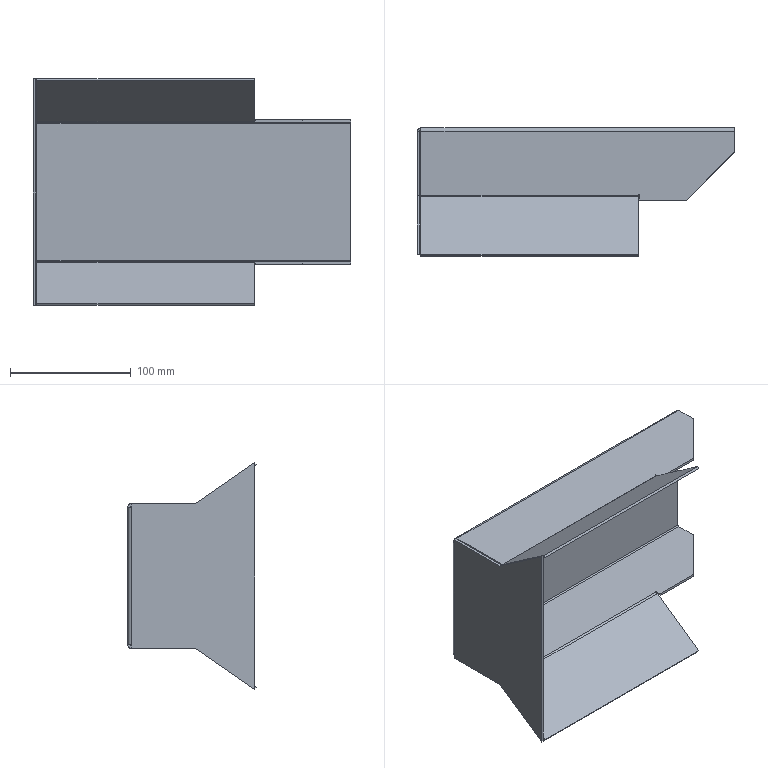Part | SolidWorks | features BaseBody 1 | 1 solid | 46 faces | box 263 x 106.293 x 188.106 mm | volume 187834 mm3 | plane 36 | cylinder 10 | commonest cylinder face diameters 2 x5 6 x5
STEP:
#1=CARTESIAN_POINT('',(-140.,-60.,118.));
#2=VERTEX_POINT('',#1);
#3=CARTESIAN_POINT('',(-100.,-20.,118.));
#4=VERTEX_POINT('',#3);
#5=CARTESIAN_POINT('',(-40.,40.,118.));
#6=DIRECTION('',(0.7071,0.7071,0.));
#7=VECTOR('',#6,1000.);
#8=LINE('',#5,#7);
#9=EDGE_CURVE('',#2,#4,#8,.T.);
#10=ORIENTED_EDGE('',*,*,#9,.T.);
#11=CARTESIAN_POINT('',(-100.,-20.,120.));
#12=VERTEX_POINT('',#11);
#13=CARTESIAN_POINT('',(-100.,-20.,272.315));
#14=DIRECTION('',(0.,0.,-1.));
#15=VECTOR('',#14,1000.);
#16=LINE('',#13,#15);
#17=EDGE_CURVE('',#12,#4,#16,.T.);
#18=ORIENTED_EDGE('',*,*,#17,.F.);
#19=CARTESIAN_POINT('',(-140.,-60.,120.));
#20=VERTEX_POINT('',#19);
#21=CARTESIAN_POINT('',(-140.,-60.,120.));
#22=DIRECTION('',(-0.7071,-0.7071,0.));
#23=VECTOR('',#22,1000.);
#24=LINE('',#21,#23);
#25=EDGE_CURVE('',#12,#20,#24,.T.);
#26=ORIENTED_EDGE('',*,*,#25,.T.);
#27=CARTESIAN_POINT('',(-140.,-60.,272.315));
#28=DIRECTION('',(0.,0.,-1.));
#29=VECTOR('',#28,1000.);
#30=LINE('',#27,#29);
#31=EDGE_CURVE('',#20,#2,#30,.T.);
#32=ORIENTED_EDGE('',*,*,#31,.T.);
#33=EDGE_LOOP('',(#10,#18,#26,#32));
#34=FACE_OUTER_BOUND('',#33,.T.);
#35=CARTESIAN_POINT('',(-140.,-60.,272.315));
#36=DIRECTION('',(-0.7071,0.7071,0.));
#37=DIRECTION('',(0.,0.,1.));
#38=AXIS2_PLACEMENT_3D('',#35,#36,#37);
#39=PLANE('',#38);
#40=ADVANCED_FACE('',(#34),#39,.F.);
#41=CARTESIAN_POINT('',(-100.,-3.,0.));
#42=VERTEX_POINT('',#41);
#43=CARTESIAN_POINT('',(-100.,0.,3.));
#44=VERTEX_POINT('',#43);
#45=CARTESIAN_POINT('',(-100.,-3.,3.));
#46=DIRECTION('',(1.,0.,0.));
#47=DIRECTION('',(0.,0.,1.));
#48=AXIS2_PLACEMENT_3D('',#45,#46,#47);
#49=CIRCLE('',#48,3.);
#50=EDGE_CURVE('',#42,#44,#49,.T.);
#51=ORIENTED_EDGE('',*,*,#50,.T.);
#52=CARTESIAN_POINT('',(-100.,0.,117.));
#53=VERTEX_POINT('',#52);
#54=CARTESIAN_POINT('',(-100.,0.,272.315));
#55=DIRECTION('',(0.,0.,-1.));
#56=VECTOR('',#55,1000.);
#57=LINE('',#54,#56);
#58=EDGE_CURVE('',#53,#44,#57,.T.);
#59=ORIENTED_EDGE('',*,*,#58,.F.);
#60=CARTESIAN_POINT('',(-100.,-3.,120.));
#61=VERTEX_POINT('',#60);
#62=CARTESIAN_POINT('',(-100.,-3.,117.));
#63=DIRECTION('',(1.,0.,0.));
#64=DIRECTION('',(0.,0.,1.));
#65=AXIS2_PLACEMENT_3D('',#62,#63,#64);
#66=CIRCLE('',#65,3.);
#67=EDGE_CURVE('',#53,#61,#66,.T.);
#68=ORIENTED_EDGE('',*,*,#67,.T.);
#69=CARTESIAN_POINT('',(-100.,-20.,120.));
#70=DIRECTION('',(0.,-1.,0.));
#71=VECTOR('',#70,1000.);
#72=LINE('',#69,#71);
#73=EDGE_CURVE('',#61,#12,#72,.T.);
#74=ORIENTED_EDGE('',*,*,#73,.T.);
#75=ORIENTED_EDGE('',*,*,#17,.T.);
#76=CARTESIAN_POINT('',(-100.,-3.,118.));
#77=VERTEX_POINT('',#76);
#78=CARTESIAN_POINT('',(-100.,0.,118.));
#79=DIRECTION('',(0.,1.,0.));
#80=VECTOR('',#79,1000.);
#81=LINE('',#78,#80);
#82=EDGE_CURVE('',#4,#77,#81,.T.);
#83=ORIENTED_EDGE('',*,*,#82,.T.);
#84=CARTESIAN_POINT('',(-100.,-2.,117.));
#85=VERTEX_POINT('',#84);
#86=CARTESIAN_POINT('',(-100.,-3.,117.));
#87=DIRECTION('',(1.,0.,0.));
#88=DIRECTION('',(0.,0.,1.));
#89=AXIS2_PLACEMENT_3D('',#86,#87,#88);
#90=CIRCLE('',#89,1.);
#91=EDGE_CURVE('',#85,#77,#90,.T.);
#92=ORIENTED_EDGE('',*,*,#91,.F.);
#93=CARTESIAN_POINT('',(-100.,-2.,3.));
#94=VERTEX_POINT('',#93);
#95=CARTESIAN_POINT('',(-100.,-2.,0.));
#96=DIRECTION('',(0.,0.,-1.));
#97=VECTOR('',#96,1000.);
#98=LINE('',#95,#97);
#99=EDGE_CURVE('',#85,#94,#98,.T.);
#100=ORIENTED_EDGE('',*,*,#99,.T.);
#101=CARTESIAN_POINT('',(-100.,-3.,2.));
#102=VERTEX_POINT('',#101);
#103=CARTESIAN_POINT('',(-100.,-3.,3.));
#104=DIRECTION('',(1.,0.,0.));
#105=DIRECTION('',(0.,0.,1.));
#106=AXIS2_PLACEMENT_3D('',#103,#104,#105);
#107=CIRCLE('',#106,1.);
#108=EDGE_CURVE('',#102,#94,#107,.T.);
#109=ORIENTED_EDGE('',*,*,#108,.F.);
#110=CARTESIAN_POINT('',(-100.,-20.,2.));
#111=VERTEX_POINT('',#110);
#112=CARTESIAN_POINT('',(-100.,0.,2.));
#113=DIRECTION('',(0.,1.,0.));
#114=VECTOR('',#113,1000.);
#115=LINE('',#112,#114);
#116=EDGE_CURVE('',#111,#102,#115,.T.);
#117=ORIENTED_EDGE('',*,*,#116,.F.);
#118=CARTESIAN_POINT('',(-100.,-20.,0.));
#119=VERTEX_POINT('',#118);
#120=CARTESIAN_POINT('',(-100.,-20.,272.315));
#121=DIRECTION('',(0.,0.,-1.));
#122=VECTOR('',#121,1000.);
#123=LINE('',#120,#122);
#124=EDGE_CURVE('',#111,#119,#123,.T.);
#125=ORIENTED_EDGE('',*,*,#124,.T.);
#126=CARTESIAN_POINT('',(-100.,-20.,0.));
#127=DIRECTION('',(0.,1.,0.));
#128=VECTOR('',#127,1000.);
#129=LINE('',#126,#128);
#130=EDGE_CURVE('',#119,#42,#129,.T.);
#131=ORIENTED_EDGE('',*,*,#130,.T.);
#132=EDGE_LOOP('',(#51,#59,#68,#74,#75,#83,#92,#100,#109,#117,#125,#131));
#133=FACE_OUTER_BOUND('',#132,.T.);
#134=CARTESIAN_POINT('',(-100.,-20.,272.315));
#135=DIRECTION('',(-1.,0.,0.));
#136=DIRECTION('',(0.,1.,0.));
#137=AXIS2_PLACEMENT_3D('',#134,#135,#136);
#138=PLANE('',#137);
#139=ADVANCED_FACE('',(#133),#138,.F.);
#140=CARTESIAN_POINT('',(-140.,-60.,2.));
#141=VERTEX_POINT('',#140);
#142=CARTESIAN_POINT('',(-140.,-60.,0.));
#143=VERTEX_POINT('',#142);
#144=CARTESIAN_POINT('',(-140.,-60.,272.315));
#145=DIRECTION('',(0.,0.,-1.));
#146=VECTOR('',#145,1000.);
#147=LINE('',#144,#146);
#148=EDGE_CURVE('',#141,#143,#147,.T.);
#149=ORIENTED_EDGE('',*,*,#148,.T.);
#150=CARTESIAN_POINT('',(-140.,-60.,0.));
#151=DIRECTION('',(0.7071,0.7071,0.));
#152=VECTOR('',#151,1000.);
#153=LINE('',#150,#152);
#154=EDGE_CURVE('',#143,#119,#153,.T.);
#155=ORIENTED_EDGE('',*,*,#154,.T.);
#156=ORIENTED_EDGE('',*,*,#124,.F.);
#157=CARTESIAN_POINT('',(-40.,40.,2.));
#158=DIRECTION('',(0.7071,0.7071,0.));
#159=VECTOR('',#158,1000.);
#160=LINE('',#157,#159);
#161=EDGE_CURVE('',#141,#111,#160,.T.);
#162=ORIENTED_EDGE('',*,*,#161,.F.);
#163=EDGE_LOOP('',(#149,#155,#156,#162));
#164=FACE_OUTER_BOUND('',#163,.T.);
#165=CARTESIAN_POINT('',(-140.,-60.,272.315));
#166=DIRECTION('',(-0.7071,0.7071,0.));
#167=DIRECTION('',(0.,0.,1.));
#168=AXIS2_PLACEMENT_3D('',#165,#166,#167);
#169=PLANE('',#168);
#170=ADVANCED_FACE('',(#164),#169,.F.);
#171=CARTESIAN_POINT('',(-360.,-56.771,120.181));
#172=VERTEX_POINT('',#171);
#173=CARTESIAN_POINT('',(-360.,-105.146,154.053));
#174=VERTEX_POINT('',#173);
#175=CARTESIAN_POINT('',(-360.,-56.771,120.181));
#176=DIRECTION('',(0.,-0.8192,0.5736));
#177=VECTOR('',#176,1000.);
#178=LINE('',#175,#177);
#179=EDGE_CURVE('',#172,#174,#178,.T.);
#180=ORIENTED_EDGE('',*,*,#179,.T.);
#181=CARTESIAN_POINT('',(-180.,-105.146,154.053));
#182=VERTEX_POINT('',#181);
#183=CARTESIAN_POINT('',(-360.,-105.146,154.053));
#184=DIRECTION('',(1.,0.,0.));
#185=VECTOR('',#184,1000.);
#186=LINE('',#183,#185);
#187=EDGE_CURVE('',#174,#182,#186,.T.);
#188=ORIENTED_EDGE('',*,*,#187,.T.);
#189=CARTESIAN_POINT('',(-180.,-56.771,120.181));
#190=VERTEX_POINT('',#189);
#191=CARTESIAN_POINT('',(-180.,-105.146,154.053));
#192=DIRECTION('',(0.,0.8192,-0.5736));
#193=VECTOR('',#192,1000.);
#194=LINE('',#191,#193);
#195=EDGE_CURVE('',#182,#190,#194,.T.);
#196=ORIENTED_EDGE('',*,*,#195,.T.);
#197=CARTESIAN_POINT('',(-180.,-56.771,120.181));
#198=DIRECTION('',(-1.,0.,0.));
#199=VECTOR('',#198,1000.);
#200=LINE('',#197,#199);
#201=EDGE_CURVE('',#190,#172,#200,.T.);
#202=ORIENTED_EDGE('',*,*,#201,.T.);
#203=EDGE_LOOP('',(#180,#188,#196,#202));
#204=FACE_OUTER_BOUND('',#203,.T.);
#205=CARTESIAN_POINT('',(0.,40.129,52.33));
#206=DIRECTION('',(0.,0.5736,0.8192));
#207=DIRECTION('',(1.,0.,0.));
#208=AXIS2_PLACEMENT_3D('',#205,#206,#207);
#209=PLANE('',#208);
#210=ADVANCED_FACE('',(#204),#209,.T.);
#211=CARTESIAN_POINT('',(-180.,-56.771,-0.1808));
#212=VERTEX_POINT('',#211);
#213=CARTESIAN_POINT('',(-180.,-105.146,-34.053));
#214=VERTEX_POINT('',#213);
#215=CARTESIAN_POINT('',(-180.,-56.771,-0.1808));
#216=DIRECTION('',(0.,-0.8192,-0.5736));
#217=VECTOR('',#216,1000.);
#218=LINE('',#215,#217);
#219=EDGE_CURVE('',#212,#214,#218,.T.);
#220=ORIENTED_EDGE('',*,*,#219,.T.);
#221=CARTESIAN_POINT('',(-360.,-105.146,-34.053));
#222=VERTEX_POINT('',#221);
#223=CARTESIAN_POINT('',(-180.,-105.146,-34.053));
#224=DIRECTION('',(-1.,0.,0.));
#225=VECTOR('',#224,1000.);
#226=LINE('',#223,#225);
#227=EDGE_CURVE('',#214,#222,#226,.T.);
#228=ORIENTED_EDGE('',*,*,#227,.T.);
#229=CARTESIAN_POINT('',(-360.,-56.771,-0.1808));
#230=VERTEX_POINT('',#229);
#231=CARTESIAN_POINT('',(-360.,-105.146,-34.053));
#232=DIRECTION('',(0.,0.8192,0.5736));
#233=VECTOR('',#232,1000.);
#234=LINE('',#231,#233);
#235=EDGE_CURVE('',#222,#230,#234,.T.);
#236=ORIENTED_EDGE('',*,*,#235,.T.);
#237=CARTESIAN_POINT('',(-360.,-56.771,-0.1808));
#238=DIRECTION('',(1.,0.,0.));
#239=VECTOR('',#238,1000.);
#240=LINE('',#237,#239);
#241=EDGE_CURVE('',#230,#212,#240,.T.);
#242=ORIENTED_EDGE('',*,*,#241,.T.);
#243=EDGE_LOOP('',(#220,#228,#236,#242));
#244=FACE_OUTER_BOUND('',#243,.T.);
#245=CARTESIAN_POINT('',(0.,-16.253,28.191));
#246=DIRECTION('',(0.,0.5736,-0.8192));
#247=DIRECTION('',(-1.,0.,0.));
#248=AXIS2_PLACEMENT_3D('',#245,#246,#247);
#249=PLANE('',#248);
#250=ADVANCED_FACE('',(#244),#249,.T.);
#251=CARTESIAN_POINT('',(-360.,-106.293,152.415));
#252=VERTEX_POINT('',#251);
#253=CARTESIAN_POINT('',(-360.,-105.146,154.053));
#254=DIRECTION('',(0.,-0.5736,-0.8192));
#255=VECTOR('',#254,1000.);
#256=LINE('',#253,#255);
#257=EDGE_CURVE('',#174,#252,#256,.T.);
#258=ORIENTED_EDGE('',*,*,#257,.T.);
#259=CARTESIAN_POINT('',(-180.,-106.293,152.415));
#260=VERTEX_POINT('',#259);
#261=CARTESIAN_POINT('',(0.,-106.293,152.415));
#262=DIRECTION('',(1.,0.,0.));
#263=VECTOR('',#262,1000.);
#264=LINE('',#261,#263);
#265=EDGE_CURVE('',#252,#260,#264,.T.);
#266=ORIENTED_EDGE('',*,*,#265,.T.);
#267=CARTESIAN_POINT('',(-180.,-106.293,152.415));
#268=DIRECTION('',(0.,0.5736,0.8192));
#269=VECTOR('',#268,1000.);
#270=LINE('',#267,#269);
#271=EDGE_CURVE('',#260,#182,#270,.T.);
#272=ORIENTED_EDGE('',*,*,#271,.T.);
#273=ORIENTED_EDGE('',*,*,#187,.F.);
#274=EDGE_LOOP('',(#258,#266,#272,#273));
#275=FACE_OUTER_BOUND('',#274,.T.);
#276=CARTESIAN_POINT('',(-360.,-106.293,152.415));
#277=DIRECTION('',(0.,0.8192,-0.5736));
#278=DIRECTION('',(-1.,0.,0.));
#279=AXIS2_PLACEMENT_3D('',#276,#277,#278);
#280=PLANE('',#279);
#281=ADVANCED_FACE('',(#275),#280,.F.);
#282=CARTESIAN_POINT('',(-360.,-56.198,120.));
#283=VERTEX_POINT('',#282);
#284=CARTESIAN_POINT('',(-360.,-56.198,121.));
#285=DIRECTION('',(1.,0.,0.));
#286=DIRECTION('',(0.,1.,0.));
#287=AXIS2_PLACEMENT_3D('',#284,#285,#286);
#288=CIRCLE('',#287,1.);
#289=EDGE_CURVE('',#172,#283,#288,.T.);
#290=ORIENTED_EDGE('',*,*,#289,.F.);
#291=ORIENTED_EDGE('',*,*,#201,.F.);
#292=CARTESIAN_POINT('',(-180.,-56.198,120.));
#293=VERTEX_POINT('',#292);
#294=CARTESIAN_POINT('',(-180.,-56.198,121.));
#295=DIRECTION('',(1.,0.,0.));
#296=DIRECTION('',(0.,1.,0.));
#297=AXIS2_PLACEMENT_3D('',#294,#295,#296);
#298=CIRCLE('',#297,1.);
#299=EDGE_CURVE('',#190,#293,#298,.T.);
#300=ORIENTED_EDGE('',*,*,#299,.T.);
#301=CARTESIAN_POINT('',(0.,-56.198,120.));
#302=DIRECTION('',(-1.,0.,0.));
#303=VECTOR('',#302,1000.);
#304=LINE('',#301,#303);
#305=EDGE_CURVE('',#293,#283,#304,.T.);
#306=ORIENTED_EDGE('',*,*,#305,.T.);
#307=EDGE_LOOP('',(#290,#291,#300,#306));
#308=FACE_OUTER_BOUND('',#307,.T.);
#309=CARTESIAN_POINT('',(-180.,-56.198,121.));
#310=DIRECTION('',(1.,0.,0.));
#311=DIRECTION('',(0.,1.,0.));
#312=AXIS2_PLACEMENT_3D('',#309,#310,#311);
#313=CYLINDRICAL_SURFACE('',#312,1.);
#314=ADVANCED_FACE('',(#308),#313,.F.);
#315=CARTESIAN_POINT('',(-180.,-56.198,0.));
#316=VERTEX_POINT('',#315);
#317=CARTESIAN_POINT('',(-180.,-56.198,-1.));
#318=DIRECTION('',(-1.,0.,0.));
#319=DIRECTION('',(0.,-1.,0.));
#320=AXIS2_PLACEMENT_3D('',#317,#318,#319);
#321=CIRCLE('',#320,1.);
#322=EDGE_CURVE('',#212,#316,#321,.T.);
#323=ORIENTED_EDGE('',*,*,#322,.F.);
#324=ORIENTED_EDGE('',*,*,#241,.F.);
#325=CARTESIAN_POINT('',(-360.,-56.198,0.));
#326=VERTEX_POINT('',#325);
#327=CARTESIAN_POINT('',(-360.,-56.198,-1.));
#328=DIRECTION('',(1.,0.,0.));
#329=DIRECTION('',(0.,-1.,0.));
#330=AXIS2_PLACEMENT_3D('',#327,#328,#329);
#331=CIRCLE('',#330,1.);
#332=EDGE_CURVE('',#326,#230,#331,.T.);
#333=ORIENTED_EDGE('',*,*,#332,.F.);
#334=CARTESIAN_POINT('',(0.,-56.198,0.));
#335=DIRECTION('',(-1.,0.,0.));
#336=VECTOR('',#335,1000.);
#337=LINE('',#334,#336);
#338=EDGE_CURVE('',#316,#326,#337,.T.);
#339=ORIENTED_EDGE('',*,*,#338,.F.);
#340=EDGE_LOOP('',(#323,#324,#333,#339));
#341=FACE_OUTER_BOUND('',#340,.T.);
#342=CARTESIAN_POINT('',(-360.,-56.198,-1.));
#343=DIRECTION('',(-1.,0.,0.));
#344=DIRECTION('',(0.,-1.,0.));
#345=AXIS2_PLACEMENT_3D('',#342,#343,#344);
#346=CYLINDRICAL_SURFACE('',#345,1.);
#347=ADVANCED_FACE('',(#341),#346,.F.);
#348=CARTESIAN_POINT('',(-180.,-106.293,-32.415));
#349=VERTEX_POINT('',#348);
#350=CARTESIAN_POINT('',(-180.,-105.146,-34.053));
#351=DIRECTION('',(0.,-0.5736,0.8192));
#352=VECTOR('',#351,1000.);
#353=LINE('',#350,#352);
#354=EDGE_CURVE('',#214,#349,#353,.T.);
#355=ORIENTED_EDGE('',*,*,#354,.T.);
#356=CARTESIAN_POINT('',(-360.,-106.293,-32.415));
#357=VERTEX_POINT('',#356);
#358=CARTESIAN_POINT('',(0.,-106.293,-32.415));
#359=DIRECTION('',(-1.,0.,0.));
#360=VECTOR('',#359,1000.);
#361=LINE('',#358,#360);
#362=EDGE_CURVE('',#349,#357,#361,.T.);
#363=ORIENTED_EDGE('',*,*,#362,.T.);
#364=CARTESIAN_POINT('',(-360.,-106.293,-32.415));
#365=DIRECTION('',(0.,0.5736,-0.8192));
#366=VECTOR('',#365,1000.);
#367=LINE('',#364,#366);
#368=EDGE_CURVE('',#357,#222,#367,.T.);
#369=ORIENTED_EDGE('',*,*,#368,.T.);
#370=ORIENTED_EDGE('',*,*,#227,.F.);
#371=EDGE_LOOP('',(#355,#363,#369,#370));
#372=FACE_OUTER_BOUND('',#371,.T.);
#373=CARTESIAN_POINT('',(-180.,-106.293,-32.415));
#374=DIRECTION('',(0.,0.8192,0.5736));
#375=DIRECTION('',(1.,0.,0.));
#376=AXIS2_PLACEMENT_3D('',#373,#374,#375);
#377=PLANE('',#376);
#378=ADVANCED_FACE('',(#372),#377,.F.);
#379=CARTESIAN_POINT('',(-179.,-55.198,120.));
#380=VERTEX_POINT('',#379);
#381=CARTESIAN_POINT('',(-180.,-55.198,120.));
#382=VERTEX_POINT('',#381);
#383=CARTESIAN_POINT('',(0.,-55.198,120.));
#384=DIRECTION('',(-1.,0.,0.));
#385=VECTOR('',#384,1000.);
#386=LINE('',#383,#385);
#387=EDGE_CURVE('',#380,#382,#386,.T.);
#388=ORIENTED_EDGE('',*,*,#387,.T.);
#389=CARTESIAN_POINT('',(-180.,-55.198,118.));
#390=VERTEX_POINT('',#389);
#391=CARTESIAN_POINT('',(-180.,-55.198,120.));
#392=DIRECTION('',(0.,0.,-1.));
#393=VECTOR('',#392,1000.);
#394=LINE('',#391,#393);
#395=EDGE_CURVE('',#382,#390,#394,.T.);
#396=ORIENTED_EDGE('',*,*,#395,.T.);
#397=CARTESIAN_POINT('',(-179.,-55.198,118.));
#398=VERTEX_POINT('',#397);
#399=CARTESIAN_POINT('',(-179.,-55.198,118.));
#400=DIRECTION('',(1.,0.,0.));
#401=VECTOR('',#400,1000.);
#402=LINE('',#399,#401);
#403=EDGE_CURVE('',#390,#398,#402,.T.);
#404=ORIENTED_EDGE('',*,*,#403,.T.);
#405=CARTESIAN_POINT('',(-179.,-55.198,120.));
#406=DIRECTION('',(0.,0.,-1.));
#407=VECTOR('',#406,1000.);
#408=LINE('',#405,#407);
#409=EDGE_CURVE('',#380,#398,#408,.T.);
#410=ORIENTED_EDGE('',*,*,#409,.F.);
#411=EDGE_LOOP('',(#388,#396,#404,#410));
#412=FACE_OUTER_BOUND('',#411,.T.);
#413=CARTESIAN_POINT('',(-179.,-55.198,120.));
#414=DIRECTION('',(0.,-1.,0.));
#415=DIRECTION('',(0.,0.,-1.));
#416=AXIS2_PLACEMENT_3D('',#413,#414,#415);
#417=PLANE('',#416);
#418=ADVANCED_FACE('',(#412),#417,.T.);
#419=ORIENTED_EDGE('',*,*,#299,.F.);
#420=ORIENTED_EDGE('',*,*,#195,.F.);
#421=ORIENTED_EDGE('',*,*,#271,.F.);
#422=CARTESIAN_POINT('',(-180.,-57.919,118.543));
#423=VERTEX_POINT('',#422);
#424=CARTESIAN_POINT('',(-180.,38.982,50.692));
#425=DIRECTION('',(0.,0.8192,-0.5736));
#426=VECTOR('',#425,1000.);
#427=LINE('',#424,#426);
#428=EDGE_CURVE('',#260,#423,#427,.T.);
#429=ORIENTED_EDGE('',*,*,#428,.T.);
#430=CARTESIAN_POINT('',(-180.,-56.198,118.));
#431=VERTEX_POINT('',#430);
#432=CARTESIAN_POINT('',(-180.,-56.198,121.));
#433=DIRECTION('',(-1.,0.,0.));
#434=DIRECTION('',(0.,1.,0.));
#435=AXIS2_PLACEMENT_3D('',#432,#433,#434);
#436=CIRCLE('',#435,3.);
#437=EDGE_CURVE('',#431,#423,#436,.T.);
#438=ORIENTED_EDGE('',*,*,#437,.F.);
#439=CARTESIAN_POINT('',(-180.,-55.198,118.));
#440=DIRECTION('',(0.,1.,0.));
#441=VECTOR('',#440,1000.);
#442=LINE('',#439,#441);
#443=EDGE_CURVE('',#431,#390,#442,.T.);
#444=ORIENTED_EDGE('',*,*,#443,.T.);
#445=ORIENTED_EDGE('',*,*,#395,.F.);
#446=CARTESIAN_POINT('',(-180.,-55.198,120.));
#447=DIRECTION('',(0.,-1.,0.));
#448=VECTOR('',#447,1000.);
#449=LINE('',#446,#448);
#450=EDGE_CURVE('',#382,#293,#449,.T.);
#451=ORIENTED_EDGE('',*,*,#450,.T.);
#452=EDGE_LOOP('',(#419,#420,#421,#429,#438,#444,#445,#451));
#453=FACE_OUTER_BOUND('',#452,.T.);
#454=CARTESIAN_POINT('',(-180.,-56.198,121.));
#455=DIRECTION('',(-1.,0.,0.));
#456=DIRECTION('',(0.,0.,1.));
#457=AXIS2_PLACEMENT_3D('',#454,#455,#456);
#458=PLANE('',#457);
#459=ADVANCED_FACE('',(#453),#458,.F.);
#460=ORIENTED_EDGE('',*,*,#428,.F.);
#461=ORIENTED_EDGE('',*,*,#265,.F.);
#462=CARTESIAN_POINT('',(-360.,-57.919,118.543));
#463=VERTEX_POINT('',#462);
#464=CARTESIAN_POINT('',(-360.,38.982,50.692));
#465=DIRECTION('',(0.,-0.8192,0.5736));
#466=VECTOR('',#465,1000.);
#467=LINE('',#464,#466);
#468=EDGE_CURVE('',#463,#252,#467,.T.);
#469=ORIENTED_EDGE('',*,*,#468,.F.);
#470=CARTESIAN_POINT('',(-180.,-57.919,118.543));
#471=DIRECTION('',(-1.,0.,0.));
#472=VECTOR('',#471,1000.);
#473=LINE('',#470,#472);
#474=EDGE_CURVE('',#423,#463,#473,.T.);
#475=ORIENTED_EDGE('',*,*,#474,.F.);
#476=EDGE_LOOP('',(#460,#461,#469,#475));
#477=FACE_OUTER_BOUND('',#476,.T.);
#478=CARTESIAN_POINT('',(0.,38.982,50.692));
#479=DIRECTION('',(0.,0.5736,0.8192));
#480=DIRECTION('',(1.,0.,0.));
#481=AXIS2_PLACEMENT_3D('',#478,#479,#480);
#482=PLANE('',#481);
#483=ADVANCED_FACE('',(#477),#482,.F.);
#484=ORIENTED_EDGE('',*,*,#25,.F.);
#485=ORIENTED_EDGE('',*,*,#73,.F.);
#486=CARTESIAN_POINT('',(-360.,-3.,120.));
#487=VERTEX_POINT('',#486);
#488=CARTESIAN_POINT('',(-360.,-3.,120.));
#489=DIRECTION('',(1.,0.,0.));
#490=VECTOR('',#489,1000.);
#491=LINE('',#488,#490);
#492=EDGE_CURVE('',#487,#61,#491,.T.);
#493=ORIENTED_EDGE('',*,*,#492,.F.);
#494=CARTESIAN_POINT('',(-360.,-60.,120.));
#495=DIRECTION('',(0.,1.,0.));
#496=VECTOR('',#495,1000.);
#497=LINE('',#494,#496);
#498=EDGE_CURVE('',#283,#487,#497,.T.);
#499=ORIENTED_EDGE('',*,*,#498,.F.);
#500=ORIENTED_EDGE('',*,*,#305,.F.);
#501=ORIENTED_EDGE('',*,*,#450,.F.);
#502=ORIENTED_EDGE('',*,*,#387,.F.);
#503=CARTESIAN_POINT('',(-179.,-60.,120.));
#504=VERTEX_POINT('',#503);
#505=CARTESIAN_POINT('',(-179.,-60.,120.));
#506=DIRECTION('',(0.,1.,0.));
#507=VECTOR('',#506,1000.);
#508=LINE('',#505,#507);
#509=EDGE_CURVE('',#504,#380,#508,.T.);
#510=ORIENTED_EDGE('',*,*,#509,.F.);
#511=CARTESIAN_POINT('',(0.,-60.,120.));
#512=DIRECTION('',(-1.,0.,0.));
#513=VECTOR('',#512,1000.);
#514=LINE('',#511,#513);
#515=EDGE_CURVE('',#20,#504,#514,.T.);
#516=ORIENTED_EDGE('',*,*,#515,.F.);
#517=EDGE_LOOP('',(#484,#485,#493,#499,#500,#501,#502,#510,#516));
#518=FACE_OUTER_BOUND('',#517,.T.);
#519=CARTESIAN_POINT('',(0.,0.,120.));
#520=DIRECTION('',(0.,0.,-1.));
#521=DIRECTION('',(0.,-1.,0.));
#522=AXIS2_PLACEMENT_3D('',#519,#520,#521);
#523=PLANE('',#522);
#524=ADVANCED_FACE('',(#518),#523,.F.);
#525=CARTESIAN_POINT('',(-363.,-3.,3.));
#526=VERTEX_POINT('',#525);
#527=CARTESIAN_POINT('',(-361.,-3.,3.));
#528=VERTEX_POINT('',#527);
#529=CARTESIAN_POINT('',(-361.,-3.,3.));
#530=DIRECTION('',(1.,0.,0.));
#531=VECTOR('',#530,1000.);
#532=LINE('',#529,#531);
#533=EDGE_CURVE('',#526,#528,#532,.T.);
#534=ORIENTED_EDGE('',*,*,#533,.F.);
#535=CARTESIAN_POINT('',(-360.,0.,3.));
#536=VERTEX_POINT('',#535);
#537=CARTESIAN_POINT('',(-360.,-3.,3.));
#538=DIRECTION('',(0.,0.,1.));
#539=DIRECTION('',(-1.,0.,0.));
#540=AXIS2_PLACEMENT_3D('',#537,#538,#539);
#541=CIRCLE('',#540,3.);
#542=EDGE_CURVE('',#536,#526,#541,.T.);
#543=ORIENTED_EDGE('',*,*,#542,.F.);
#544=CARTESIAN_POINT('',(-360.,-2.,3.));
#545=VERTEX_POINT('',#544);
#546=CARTESIAN_POINT('',(-360.,-3.,3.));
#547=DIRECTION('',(0.,1.,0.));
#548=VECTOR('',#547,1000.);
#549=LINE('',#546,#548);
#550=EDGE_CURVE('',#545,#536,#549,.T.);
#551=ORIENTED_EDGE('',*,*,#550,.F.);
#552=CARTESIAN_POINT('',(-360.,-3.,3.));
#553=DIRECTION('',(0.,0.,-1.));
#554=DIRECTION('',(-1.,0.,0.));
#555=AXIS2_PLACEMENT_3D('',#552,#553,#554);
#556=CIRCLE('',#555,1.);
#557=EDGE_CURVE('',#528,#545,#556,.T.);
#558=ORIENTED_EDGE('',*,*,#557,.F.);
#559=EDGE_LOOP('',(#534,#543,#551,#558));
#560=FACE_OUTER_BOUND('',#559,.T.);
#561=CARTESIAN_POINT('',(-360.,-3.,3.));
#562=DIRECTION('',(0.,0.,1.));
#563=DIRECTION('',(1.,0.,0.));
#564=AXIS2_PLACEMENT_3D('',#561,#562,#563);
#565=PLANE('',#564);
#566=ADVANCED_FACE('',(#560),#565,.F.);
#567=CARTESIAN_POINT('',(-360.,-2.,117.));
#568=VERTEX_POINT('',#567);
#569=CARTESIAN_POINT('',(-360.,0.,117.));
#570=VERTEX_POINT('',#569);
#571=CARTESIAN_POINT('',(-360.,-3.,117.));
#572=DIRECTION('',(0.,1.,0.));
#573=VECTOR('',#572,1000.);
#574=LINE('',#571,#573);
#575=EDGE_CURVE('',#568,#570,#574,.T.);
#576=ORIENTED_EDGE('',*,*,#575,.T.);
#577=CARTESIAN_POINT('',(-363.,-3.,117.));
#578=VERTEX_POINT('',#577);
#579=CARTESIAN_POINT('',(-360.,-3.,117.));
#580=DIRECTION('',(0.,0.,-1.));
#581=DIRECTION('',(-1.,0.,0.));
#582=AXIS2_PLACEMENT_3D('',#579,#580,#581);
#583=CIRCLE('',#582,3.);
#584=EDGE_CURVE('',#578,#570,#583,.T.);
#585=ORIENTED_EDGE('',*,*,#584,.F.);
#586=CARTESIAN_POINT('',(-361.,-3.,117.));
#587=VERTEX_POINT('',#586);
#588=CARTESIAN_POINT('',(-361.,-3.,117.));
#589=DIRECTION('',(-1.,0.,0.));
#590=VECTOR('',#589,1000.);
#591=LINE('',#588,#590);
#592=EDGE_CURVE('',#587,#578,#591,.T.);
#593=ORIENTED_EDGE('',*,*,#592,.F.);
#594=CARTESIAN_POINT('',(-360.,-3.,117.));
#595=DIRECTION('',(0.,0.,-1.));
#596=DIRECTION('',(-1.,0.,0.));
#597=AXIS2_PLACEMENT_3D('',#594,#595,#596);
#598=CIRCLE('',#597,1.);
#599=EDGE_CURVE('',#587,#568,#598,.T.);
#600=ORIENTED_EDGE('',*,*,#599,.T.);
#601=EDGE_LOOP('',(#576,#585,#593,#600));
#602=FACE_OUTER_BOUND('',#601,.T.);
#603=CARTESIAN_POINT('',(-360.,-3.,117.));
#604=DIRECTION('',(0.,0.,1.));
#605=DIRECTION('',(1.,0.,0.));
#606=AXIS2_PLACEMENT_3D('',#603,#604,#605);
#607=PLANE('',#606);
#608=ADVANCED_FACE('',(#602),#607,.T.);
#609=CARTESIAN_POINT('',(-363.,-3.,0.));
#610=VERTEX_POINT('',#609);
#611=CARTESIAN_POINT('',(-363.,-56.198,0.));
#612=VERTEX_POINT('',#611);
#613=CARTESIAN_POINT('',(-363.,-56.198,0.));
#614=DIRECTION('',(0.,-1.,0.));
#615=VECTOR('',#614,1000.);
#616=LINE('',#613,#615);
#617=EDGE_CURVE('',#610,#612,#616,.T.);
#618=ORIENTED_EDGE('',*,*,#617,.T.);
#619=CARTESIAN_POINT('',(-363.,-105.146,-34.053));
#620=VERTEX_POINT('',#619);
#621=CARTESIAN_POINT('',(-363.,-56.198,0.));
#622=DIRECTION('',(0.,-0.8209,-0.5711));
#623=VECTOR('',#622,1000.);
#624=LINE('',#621,#623);
#625=EDGE_CURVE('',#612,#620,#624,.T.);
#626=ORIENTED_EDGE('',*,*,#625,.T.);
#627=CARTESIAN_POINT('',(-363.,-105.146,154.053));
#628=VERTEX_POINT('',#627);
#629=CARTESIAN_POINT('',(-363.,-105.146,154.053));
#630=DIRECTION('',(0.,0.,1.));
#631=VECTOR('',#630,1000.);
#632=LINE('',#629,#631);
#633=EDGE_CURVE('',#620,#628,#632,.T.);
#634=ORIENTED_EDGE('',*,*,#633,.T.);
#635=CARTESIAN_POINT('',(-363.,-56.198,120.));
#636=VERTEX_POINT('',#635);
#637=CARTESIAN_POINT('',(-363.,-56.198,120.));
#638=DIRECTION('',(0.,0.8209,-0.5711));
#639=VECTOR('',#638,1000.);
#640=LINE('',#637,#639);
#641=EDGE_CURVE('',#628,#636,#640,.T.);
#642=ORIENTED_EDGE('',*,*,#641,.T.);
#643=CARTESIAN_POINT('',(-363.,-3.,120.));
#644=VERTEX_POINT('',#643);
#645=CARTESIAN_POINT('',(-363.,-2.,120.));
#646=DIRECTION('',(0.,1.,0.));
#647=VECTOR('',#646,1000.);
#648=LINE('',#645,#647);
#649=EDGE_CURVE('',#636,#644,#648,.T.);
#650=ORIENTED_EDGE('',*,*,#649,.T.);
#651=CARTESIAN_POINT('',(-363.,-3.,120.));
#652=DIRECTION('',(0.,0.,1.));
#653=VECTOR('',#652,1000.);
#654=LINE('',#651,#653);
#655=EDGE_CURVE('',#578,#644,#654,.T.);
#656=ORIENTED_EDGE('',*,*,#655,.F.);
#657=CARTESIAN_POINT('',(-363.,-3.,3.));
#658=DIRECTION('',(0.,0.,1.));
#659=VECTOR('',#658,1000.);
#660=LINE('',#657,#659);
#661=EDGE_CURVE('',#526,#578,#660,.T.);
#662=ORIENTED_EDGE('',*,*,#661,.F.);
#663=CARTESIAN_POINT('',(-363.,-3.,120.));
#664=DIRECTION('',(0.,0.,1.));
#665=VECTOR('',#664,1000.);
#666=LINE('',#663,#665);
#667=EDGE_CURVE('',#610,#526,#666,.T.);
#668=ORIENTED_EDGE('',*,*,#667,.F.);
#669=EDGE_LOOP('',(#618,#626,#634,#642,#650,#656,#662,#668));
#670=FACE_OUTER_BOUND('',#669,.T.);
#671=CARTESIAN_POINT('',(-363.,0.,0.));
#672=DIRECTION('',(1.,0.,0.));
#673=DIRECTION('',(0.,-1.,0.));
#674=AXIS2_PLACEMENT_3D('',#671,#672,#673);
#675=PLANE('',#674);
#676=ADVANCED_FACE('',(#670),#675,.F.);
#677=CARTESIAN_POINT('',(-180.,-55.198,2.));
#678=VERTEX_POINT('',#677);
#679=CARTESIAN_POINT('',(-180.,-55.198,0.));
#680=VERTEX_POINT('',#679);
#681=CARTESIAN_POINT('',(-180.,-55.198,0.));
#682=DIRECTION('',(0.,0.,-1.));
#683=VECTOR('',#682,1000.);
#684=LINE('',#681,#683);
#685=EDGE_CURVE('',#678,#680,#684,.T.);
#686=ORIENTED_EDGE('',*,*,#685,.T.);
#687=CARTESIAN_POINT('',(-179.,-55.198,0.));
#688=VERTEX_POINT('',#687);
#689=CARTESIAN_POINT('',(0.,-55.198,0.));
#690=DIRECTION('',(-1.,0.,0.));
#691=VECTOR('',#690,1000.);
#692=LINE('',#689,#691);
#693=EDGE_CURVE('',#688,#680,#692,.T.);
#694=ORIENTED_EDGE('',*,*,#693,.F.);
#695=CARTESIAN_POINT('',(-179.,-55.198,2.));
#696=VERTEX_POINT('',#695);
#697=CARTESIAN_POINT('',(-179.,-55.198,0.));
#698=DIRECTION('',(0.,0.,-1.));
#699=VECTOR('',#698,1000.);
#700=LINE('',#697,#699);
#701=EDGE_CURVE('',#696,#688,#700,.T.);
#702=ORIENTED_EDGE('',*,*,#701,.F.);
#703=CARTESIAN_POINT('',(-180.,-55.198,2.));
#704=DIRECTION('',(-1.,0.,0.));
#705=VECTOR('',#704,1000.);
#706=LINE('',#703,#705);
#707=EDGE_CURVE('',#696,#678,#706,.T.);
#708=ORIENTED_EDGE('',*,*,#707,.T.);
#709=EDGE_LOOP('',(#686,#694,#702,#708));
#710=FACE_OUTER_BOUND('',#709,.T.);
#711=CARTESIAN_POINT('',(-180.,-55.198,0.));
#712=DIRECTION('',(0.,-1.,0.));
#713=DIRECTION('',(0.,0.,-1.));
#714=AXIS2_PLACEMENT_3D('',#711,#712,#713);
#715=PLANE('',#714);
#716=ADVANCED_FACE('',(#710),#715,.T.);
#717=ORIENTED_EDGE('',*,*,#130,.F.);
#718=ORIENTED_EDGE('',*,*,#154,.F.);
#719=CARTESIAN_POINT('',(-179.,-60.,0.));
#720=VERTEX_POINT('',#719);
#721=CARTESIAN_POINT('',(0.,-60.,0.));
#722=DIRECTION('',(1.,0.,0.));
#723=VECTOR('',#722,1000.);
#724=LINE('',#721,#723);
#725=EDGE_CURVE('',#720,#143,#724,.T.);
#726=ORIENTED_EDGE('',*,*,#725,.F.);
#727=CARTESIAN_POINT('',(-179.,-55.198,0.));
#728=DIRECTION('',(0.,-1.,0.));
#729=VECTOR('',#728,1000.);
#730=LINE('',#727,#729);
#731=EDGE_CURVE('',#688,#720,#730,.T.);
#732=ORIENTED_EDGE('',*,*,#731,.F.);
#733=ORIENTED_EDGE('',*,*,#693,.T.);
#734=CARTESIAN_POINT('',(-180.,0.,0.));
#735=DIRECTION('',(0.,-1.,0.));
#736=VECTOR('',#735,1000.);
#737=LINE('',#734,#736);
#738=EDGE_CURVE('',#680,#316,#737,.T.);
#739=ORIENTED_EDGE('',*,*,#738,.T.);
#740=ORIENTED_EDGE('',*,*,#338,.T.);
#741=CARTESIAN_POINT('',(-360.,-3.,0.));
#742=VERTEX_POINT('',#741);
#743=CARTESIAN_POINT('',(-360.,-60.,0.));
#744=DIRECTION('',(0.,-1.,0.));
#745=VECTOR('',#744,1000.);
#746=LINE('',#743,#745);
#747=EDGE_CURVE('',#742,#326,#746,.T.);
#748=ORIENTED_EDGE('',*,*,#747,.F.);
#749=CARTESIAN_POINT('',(0.,-3.,0.));
#750=DIRECTION('',(-1.,0.,0.));
#751=VECTOR('',#750,1000.);
#752=LINE('',#749,#751);
#753=EDGE_CURVE('',#42,#742,#752,.T.);
#754=ORIENTED_EDGE('',*,*,#753,.F.);
#755=EDGE_LOOP('',(#717,#718,#726,#732,#733,#739,#740,#748,#754));
#756=FACE_OUTER_BOUND('',#755,.T.);
#757=CARTESIAN_POINT('',(0.,0.,0.));
#758=DIRECTION('',(0.,0.,-1.));
#759=DIRECTION('',(-1.,0.,0.));
#760=AXIS2_PLACEMENT_3D('',#757,#758,#759);
#761=PLANE('',#760);
#762=ADVANCED_FACE('',(#756),#761,.T.);
#763=CARTESIAN_POINT('',(-360.,-57.919,1.457));
#764=VERTEX_POINT('',#763);
#765=CARTESIAN_POINT('',(-360.,-17.4,29.829));
#766=DIRECTION('',(0.,0.8192,0.5736));
#767=VECTOR('',#766,1000.);
#768=LINE('',#765,#767);
#769=EDGE_CURVE('',#357,#764,#768,.T.);
#770=ORIENTED_EDGE('',*,*,#769,.F.);
#771=ORIENTED_EDGE('',*,*,#362,.F.);
#772=CARTESIAN_POINT('',(-180.,-57.919,1.457));
#773=VERTEX_POINT('',#772);
#774=CARTESIAN_POINT('',(-180.,-17.4,29.829));
#775=DIRECTION('',(0.,-0.8192,-0.5736));
#776=VECTOR('',#775,1000.);
#777=LINE('',#774,#776);
#778=EDGE_CURVE('',#773,#349,#777,.T.);
#779=ORIENTED_EDGE('',*,*,#778,.F.);
#780=CARTESIAN_POINT('',(-360.,-57.919,1.457));
#781=DIRECTION('',(1.,0.,0.));
#782=VECTOR('',#781,1000.);
#783=LINE('',#780,#782);
#784=EDGE_CURVE('',#764,#773,#783,.T.);
#785=ORIENTED_EDGE('',*,*,#784,.F.);
#786=EDGE_LOOP('',(#770,#771,#779,#785));
#787=FACE_OUTER_BOUND('',#786,.T.);
#788=CARTESIAN_POINT('',(0.,-17.4,29.829));
#789=DIRECTION('',(0.,0.5736,-0.8192));
#790=DIRECTION('',(-1.,0.,0.));
#791=AXIS2_PLACEMENT_3D('',#788,#789,#790);
#792=PLANE('',#791);
#793=ADVANCED_FACE('',(#787),#792,.F.);
#794=ORIENTED_EDGE('',*,*,#322,.T.);
#795=ORIENTED_EDGE('',*,*,#738,.F.);
#796=ORIENTED_EDGE('',*,*,#685,.F.);
#797=CARTESIAN_POINT('',(-180.,-56.198,2.));
#798=VERTEX_POINT('',#797);
#799=CARTESIAN_POINT('',(-180.,-56.198,2.));
#800=DIRECTION('',(0.,-1.,0.));
#801=VECTOR('',#800,1000.);
#802=LINE('',#799,#801);
#803=EDGE_CURVE('',#678,#798,#802,.T.);
#804=ORIENTED_EDGE('',*,*,#803,.T.);
#805=CARTESIAN_POINT('',(-180.,-56.198,-1.));
#806=DIRECTION('',(-1.,0.,0.));
#807=DIRECTION('',(0.,-1.,0.));
#808=AXIS2_PLACEMENT_3D('',#805,#806,#807);
#809=CIRCLE('',#808,3.);
#810=EDGE_CURVE('',#773,#798,#809,.T.);
#811=ORIENTED_EDGE('',*,*,#810,.F.);
#812=ORIENTED_EDGE('',*,*,#778,.T.);
#813=ORIENTED_EDGE('',*,*,#354,.F.);
#814=ORIENTED_EDGE('',*,*,#219,.F.);
#815=EDGE_LOOP('',(#794,#795,#796,#804,#811,#812,#813,#814));
#816=FACE_OUTER_BOUND('',#815,.T.);
#817=CARTESIAN_POINT('',(-180.,-56.198,-1.));
#818=DIRECTION('',(1.,0.,0.));
#819=DIRECTION('',(0.,1.,0.));
#820=AXIS2_PLACEMENT_3D('',#817,#818,#819);
#821=PLANE('',#820);
#822=ADVANCED_FACE('',(#816),#821,.T.);
#823=ORIENTED_EDGE('',*,*,#661,.T.);
#824=ORIENTED_EDGE('',*,*,#584,.T.);
#825=CARTESIAN_POINT('',(-360.,0.,0.));
#826=DIRECTION('',(0.,0.,-1.));
#827=VECTOR('',#826,1000.);
#828=LINE('',#825,#827);
#829=EDGE_CURVE('',#570,#536,#828,.T.);
#830=ORIENTED_EDGE('',*,*,#829,.T.);
#831=ORIENTED_EDGE('',*,*,#542,.T.);
#832=EDGE_LOOP('',(#823,#824,#830,#831));
#833=FACE_OUTER_BOUND('',#832,.T.);
#834=CARTESIAN_POINT('',(-360.,-3.,3.));
#835=DIRECTION('',(0.,0.,-1.));
#836=DIRECTION('',(-1.,0.,0.));
#837=AXIS2_PLACEMENT_3D('',#834,#835,#836);
#838=CYLINDRICAL_SURFACE('',#837,3.);
#839=ADVANCED_FACE('',(#833),#838,.T.);
#840=ORIENTED_EDGE('',*,*,#50,.F.);
#841=ORIENTED_EDGE('',*,*,#753,.T.);
#842=CARTESIAN_POINT('',(-360.,-3.,3.));
#843=DIRECTION('',(1.,0.,0.));
#844=DIRECTION('',(0.,0.,-1.));
#845=AXIS2_PLACEMENT_3D('',#842,#843,#844);
#846=CIRCLE('',#845,3.);
#847=EDGE_CURVE('',#742,#536,#846,.T.);
#848=ORIENTED_EDGE('',*,*,#847,.T.);
#849=CARTESIAN_POINT('',(0.,0.,3.));
#850=DIRECTION('',(1.,0.,0.));
#851=VECTOR('',#850,1000.);
#852=LINE('',#849,#851);
#853=EDGE_CURVE('',#536,#44,#852,.T.);
#854=ORIENTED_EDGE('',*,*,#853,.T.);
#855=EDGE_LOOP('',(#840,#841,#848,#854));
#856=FACE_OUTER_BOUND('',#855,.T.);
#857=CARTESIAN_POINT('',(0.,-3.,3.));
#858=DIRECTION('',(1.,0.,0.));
#859=DIRECTION('',(0.,0.,-1.));
#860=AXIS2_PLACEMENT_3D('',#857,#858,#859);
#861=CYLINDRICAL_SURFACE('',#860,3.);
#862=ADVANCED_FACE('',(#856),#861,.T.);
#863=ORIENTED_EDGE('',*,*,#67,.F.);
#864=CARTESIAN_POINT('',(0.,0.,117.));
#865=DIRECTION('',(-1.,0.,0.));
#866=VECTOR('',#865,1000.);
#867=LINE('',#864,#866);
#868=EDGE_CURVE('',#53,#570,#867,.T.);
#869=ORIENTED_EDGE('',*,*,#868,.T.);
#870=CARTESIAN_POINT('',(-360.,-3.,117.));
#871=DIRECTION('',(1.,0.,0.));
#872=DIRECTION('',(0.,0.,1.));
#873=AXIS2_PLACEMENT_3D('',#870,#871,#872);
#874=CIRCLE('',#873,3.);
#875=EDGE_CURVE('',#570,#487,#874,.T.);
#876=ORIENTED_EDGE('',*,*,#875,.T.);
#877=ORIENTED_EDGE('',*,*,#492,.T.);
#878=EDGE_LOOP('',(#863,#869,#876,#877));
#879=FACE_OUTER_BOUND('',#878,.T.);
#880=CARTESIAN_POINT('',(-360.,-3.,117.));
#881=DIRECTION('',(-1.,0.,0.));
#882=DIRECTION('',(0.,0.,1.));
#883=AXIS2_PLACEMENT_3D('',#880,#881,#882);
#884=CYLINDRICAL_SURFACE('',#883,3.);
#885=ADVANCED_FACE('',(#879),#884,.T.);
#886=ORIENTED_EDGE('',*,*,#31,.F.);
#887=ORIENTED_EDGE('',*,*,#515,.T.);
#888=CARTESIAN_POINT('',(-179.,-60.,118.));
#889=VERTEX_POINT('',#888);
#890=CARTESIAN_POINT('',(-179.,-60.,120.));
#891=DIRECTION('',(0.,0.,1.));
#892=VECTOR('',#891,1000.);
#893=LINE('',#890,#892);
#894=EDGE_CURVE('',#889,#504,#893,.T.);
#895=ORIENTED_EDGE('',*,*,#894,.F.);
#896=CARTESIAN_POINT('',(0.,-60.,118.));
#897=DIRECTION('',(-1.,0.,0.));
#898=VECTOR('',#897,1000.);
#899=LINE('',#896,#898);
#900=EDGE_CURVE('',#2,#889,#899,.T.);
#901=ORIENTED_EDGE('',*,*,#900,.F.);
#902=EDGE_LOOP('',(#886,#887,#895,#901));
#903=FACE_OUTER_BOUND('',#902,.T.);
#904=CARTESIAN_POINT('',(0.,-60.,120.));
#905=DIRECTION('',(0.,-1.,0.));
#906=DIRECTION('',(-1.,0.,0.));
#907=AXIS2_PLACEMENT_3D('',#904,#905,#906);
#908=PLANE('',#907);
#909=ADVANCED_FACE('',(#903),#908,.T.);
#910=ORIENTED_EDGE('',*,*,#509,.T.);
#911=ORIENTED_EDGE('',*,*,#409,.T.);
#912=CARTESIAN_POINT('',(-179.,0.,118.));
#913=DIRECTION('',(0.,1.,0.));
#914=VECTOR('',#913,1000.);
#915=LINE('',#912,#914);
#916=EDGE_CURVE('',#889,#398,#915,.T.);
#917=ORIENTED_EDGE('',*,*,#916,.F.);
#918=ORIENTED_EDGE('',*,*,#894,.T.);
#919=EDGE_LOOP('',(#910,#911,#917,#918));
#920=FACE_OUTER_BOUND('',#919,.T.);
#921=CARTESIAN_POINT('',(-179.,-60.,120.));
#922=DIRECTION('',(-1.,0.,0.));
#923=DIRECTION('',(0.,0.,1.));
#924=AXIS2_PLACEMENT_3D('',#921,#922,#923);
#925=PLANE('',#924);
#926=ADVANCED_FACE('',(#920),#925,.T.);
#927=ORIENTED_EDGE('',*,*,#474,.T.);
#928=CARTESIAN_POINT('',(-360.,-56.198,118.));
#929=VERTEX_POINT('',#928);
#930=CARTESIAN_POINT('',(-360.,-56.198,121.));
#931=DIRECTION('',(1.,0.,0.));
#932=DIRECTION('',(0.,1.,0.));
#933=AXIS2_PLACEMENT_3D('',#930,#931,#932);
#934=CIRCLE('',#933,3.);
#935=EDGE_CURVE('',#463,#929,#934,.T.);
#936=ORIENTED_EDGE('',*,*,#935,.T.);
#937=CARTESIAN_POINT('',(0.,-56.198,118.));
#938=DIRECTION('',(-1.,0.,0.));
#939=VECTOR('',#938,1000.);
#940=LINE('',#937,#939);
#941=EDGE_CURVE('',#431,#929,#940,.T.);
#942=ORIENTED_EDGE('',*,*,#941,.F.);
#943=ORIENTED_EDGE('',*,*,#437,.T.);
#944=EDGE_LOOP('',(#927,#936,#942,#943));
#945=FACE_OUTER_BOUND('',#944,.T.);
#946=CARTESIAN_POINT('',(-180.,-56.198,121.));
#947=DIRECTION('',(1.,0.,0.));
#948=DIRECTION('',(0.,1.,0.));
#949=AXIS2_PLACEMENT_3D('',#946,#947,#948);
#950=CYLINDRICAL_SURFACE('',#949,3.);
#951=ADVANCED_FACE('',(#945),#950,.T.);
#952=ORIENTED_EDGE('',*,*,#498,.T.);
#953=ORIENTED_EDGE('',*,*,#875,.F.);
#954=ORIENTED_EDGE('',*,*,#575,.F.);
#955=CARTESIAN_POINT('',(-360.,-3.,118.));
#956=VERTEX_POINT('',#955);
#957=CARTESIAN_POINT('',(-360.,-3.,117.));
#958=DIRECTION('',(-1.,0.,0.));
#959=DIRECTION('',(0.,0.,1.));
#960=AXIS2_PLACEMENT_3D('',#957,#958,#959);
#961=CIRCLE('',#960,1.);
#962=EDGE_CURVE('',#956,#568,#961,.T.);
#963=ORIENTED_EDGE('',*,*,#962,.F.);
#964=CARTESIAN_POINT('',(-360.,0.,118.));
#965=DIRECTION('',(0.,1.,0.));
#966=VECTOR('',#965,1000.);
#967=LINE('',#964,#966);
#968=EDGE_CURVE('',#929,#956,#967,.T.);
#969=ORIENTED_EDGE('',*,*,#968,.F.);
#970=ORIENTED_EDGE('',*,*,#935,.F.);
#971=ORIENTED_EDGE('',*,*,#468,.T.);
#972=ORIENTED_EDGE('',*,*,#257,.F.);
#973=ORIENTED_EDGE('',*,*,#179,.F.);
#974=ORIENTED_EDGE('',*,*,#289,.T.);
#975=EDGE_LOOP('',(#952,#953,#954,#963,#969,#970,#971,#972,#973,#974));
#976=FACE_OUTER_BOUND('',#975,.T.);
#977=CARTESIAN_POINT('',(-360.,-60.,120.));
#978=DIRECTION('',(-1.,0.,0.));
#979=DIRECTION('',(0.,1.,0.));
#980=AXIS2_PLACEMENT_3D('',#977,#978,#979);
#981=PLANE('',#980);
#982=ADVANCED_FACE('',(#976),#981,.T.);
#983=CARTESIAN_POINT('',(-361.,-56.198,0.));
#984=VERTEX_POINT('',#983);
#985=CARTESIAN_POINT('',(-361.,-3.,0.));
#986=VERTEX_POINT('',#985);
#987=CARTESIAN_POINT('',(-361.,0.,0.));
#988=DIRECTION('',(0.,1.,0.));
#989=VECTOR('',#988,1000.);
#990=LINE('',#987,#989);
#991=EDGE_CURVE('',#984,#986,#990,.T.);
#992=ORIENTED_EDGE('',*,*,#991,.F.);
#993=CARTESIAN_POINT('',(-363.,-56.198,0.));
#994=DIRECTION('',(-1.,0.,0.));
#995=VECTOR('',#994,1000.);
#996=LINE('',#993,#995);
#997=EDGE_CURVE('',#984,#612,#996,.T.);
#998=ORIENTED_EDGE('',*,*,#997,.T.);
#999=ORIENTED_EDGE('',*,*,#617,.F.);
#1000=CARTESIAN_POINT('',(-361.,-3.,0.));
#1001=DIRECTION('',(-1.,0.,0.));
#1002=VECTOR('',#1001,1000.);
#1003=LINE('',#1000,#1002);
#1004=EDGE_CURVE('',#986,#610,#1003,.T.);
#1005=ORIENTED_EDGE('',*,*,#1004,.F.);
#1006=EDGE_LOOP('',(#992,#998,#999,#1005));
#1007=FACE_OUTER_BOUND('',#1006,.T.);
#1008=CARTESIAN_POINT('',(-363.,-56.198,0.));
#1009=DIRECTION('',(0.,0.,1.));
#1010=DIRECTION('',(0.,-1.,0.));
#1011=AXIS2_PLACEMENT_3D('',#1008,#1009,#1010);
#1012=PLANE('',#1011);
#1013=ADVANCED_FACE('',(#1007),#1012,.F.);
#1014=ORIENTED_EDGE('',*,*,#1004,.T.);
#1015=ORIENTED_EDGE('',*,*,#667,.T.);
#1016=ORIENTED_EDGE('',*,*,#533,.T.);
#1017=CARTESIAN_POINT('',(-361.,-3.,0.));
#1018=DIRECTION('',(0.,0.,1.));
#1019=VECTOR('',#1018,1000.);
#1020=LINE('',#1017,#1019);
#1021=EDGE_CURVE('',#986,#528,#1020,.T.);
#1022=ORIENTED_EDGE('',*,*,#1021,.F.);
#1023=EDGE_LOOP('',(#1014,#1015,#1016,#1022));
#1024=FACE_OUTER_BOUND('',#1023,.T.);
#1025=CARTESIAN_POINT('',(-361.,-3.,120.));
#1026=DIRECTION('',(0.,1.,0.));
#1027=DIRECTION('',(1.,0.,0.));
#1028=AXIS2_PLACEMENT_3D('',#1025,#1026,#1027);
#1029=PLANE('',#1028);
#1030=ADVANCED_FACE('',(#1024),#1029,.T.);
#1031=ORIENTED_EDGE('',*,*,#655,.T.);
#1032=CARTESIAN_POINT('',(-361.,-3.,120.));
#1033=VERTEX_POINT('',#1032);
#1034=CARTESIAN_POINT('',(-363.,-3.,120.));
#1035=DIRECTION('',(1.,0.,0.));
#1036=VECTOR('',#1035,1000.);
#1037=LINE('',#1034,#1036);
#1038=EDGE_CURVE('',#644,#1033,#1037,.T.);
#1039=ORIENTED_EDGE('',*,*,#1038,.T.);
#1040=CARTESIAN_POINT('',(-361.,-3.,0.));
#1041=DIRECTION('',(0.,0.,1.));
#1042=VECTOR('',#1041,1000.);
#1043=LINE('',#1040,#1042);
#1044=EDGE_CURVE('',#587,#1033,#1043,.T.);
#1045=ORIENTED_EDGE('',*,*,#1044,.F.);
#1046=ORIENTED_EDGE('',*,*,#592,.T.);
#1047=EDGE_LOOP('',(#1031,#1039,#1045,#1046));
#1048=FACE_OUTER_BOUND('',#1047,.T.);
#1049=CARTESIAN_POINT('',(-361.,-3.,120.));
#1050=DIRECTION('',(0.,1.,0.));
#1051=DIRECTION('',(1.,0.,0.));
#1052=AXIS2_PLACEMENT_3D('',#1049,#1050,#1051);
#1053=PLANE('',#1052);
#1054=ADVANCED_FACE('',(#1048),#1053,.T.);
#1055=ORIENTED_EDGE('',*,*,#649,.F.);
#1056=CARTESIAN_POINT('',(-361.,-56.198,120.));
#1057=VERTEX_POINT('',#1056);
#1058=CARTESIAN_POINT('',(-363.,-56.198,120.));
#1059=DIRECTION('',(1.,0.,0.));
#1060=VECTOR('',#1059,1000.);
#1061=LINE('',#1058,#1060);
#1062=EDGE_CURVE('',#636,#1057,#1061,.T.);
#1063=ORIENTED_EDGE('',*,*,#1062,.T.);
#1064=CARTESIAN_POINT('',(-361.,0.,120.));
#1065=DIRECTION('',(0.,-1.,0.));
#1066=VECTOR('',#1065,1000.);
#1067=LINE('',#1064,#1066);
#1068=EDGE_CURVE('',#1033,#1057,#1067,.T.);
#1069=ORIENTED_EDGE('',*,*,#1068,.F.);
#1070=ORIENTED_EDGE('',*,*,#1038,.F.);
#1071=EDGE_LOOP('',(#1055,#1063,#1069,#1070));
#1072=FACE_OUTER_BOUND('',#1071,.T.);
#1073=CARTESIAN_POINT('',(-363.,-2.,120.));
#1074=DIRECTION('',(0.,0.,-1.));
#1075=DIRECTION('',(-1.,0.,0.));
#1076=AXIS2_PLACEMENT_3D('',#1073,#1074,#1075);
#1077=PLANE('',#1076);
#1078=ADVANCED_FACE('',(#1072),#1077,.F.);
#1079=ORIENTED_EDGE('',*,*,#1062,.F.);
#1080=ORIENTED_EDGE('',*,*,#641,.F.);
#1081=CARTESIAN_POINT('',(-361.,-105.146,154.053));
#1082=VERTEX_POINT('',#1081);
#1083=CARTESIAN_POINT('',(-363.,-105.146,154.053));
#1084=DIRECTION('',(1.,0.,0.));
#1085=VECTOR('',#1084,1000.);
#1086=LINE('',#1083,#1085);
#1087=EDGE_CURVE('',#628,#1082,#1086,.T.);
#1088=ORIENTED_EDGE('',*,*,#1087,.T.);
#1089=CARTESIAN_POINT('',(-361.,-56.198,120.));
#1090=DIRECTION('',(0.,-0.8209,0.5711));
#1091=VECTOR('',#1090,1000.);
#1092=LINE('',#1089,#1091);
#1093=EDGE_CURVE('',#1057,#1082,#1092,.T.);
#1094=ORIENTED_EDGE('',*,*,#1093,.F.);
#1095=EDGE_LOOP('',(#1079,#1080,#1088,#1094));
#1096=FACE_OUTER_BOUND('',#1095,.T.);
#1097=CARTESIAN_POINT('',(-363.,-56.198,120.));
#1098=DIRECTION('',(0.,-0.5711,-0.8209));
#1099=DIRECTION('',(0.,-0.8209,0.5711));
#1100=AXIS2_PLACEMENT_3D('',#1097,#1098,#1099);
#1101=PLANE('',#1100);
#1102=ADVANCED_FACE('',(#1096),#1101,.F.);
#1103=ORIENTED_EDGE('',*,*,#1087,.F.);
#1104=ORIENTED_EDGE('',*,*,#633,.F.);
#1105=CARTESIAN_POINT('',(-361.,-105.146,-34.053));
#1106=VERTEX_POINT('',#1105);
#1107=CARTESIAN_POINT('',(-363.,-105.146,-34.053));
#1108=DIRECTION('',(1.,0.,0.));
#1109=VECTOR('',#1108,1000.);
#1110=LINE('',#1107,#1109);
#1111=EDGE_CURVE('',#620,#1106,#1110,.T.);
#1112=ORIENTED_EDGE('',*,*,#1111,.T.);
#1113=CARTESIAN_POINT('',(-361.,-105.146,0.));
#1114=DIRECTION('',(0.,0.,-1.));
#1115=VECTOR('',#1114,1000.);
#1116=LINE('',#1113,#1115);
#1117=EDGE_CURVE('',#1082,#1106,#1116,.T.);
#1118=ORIENTED_EDGE('',*,*,#1117,.F.);
#1119=EDGE_LOOP('',(#1103,#1104,#1112,#1118));
#1120=FACE_OUTER_BOUND('',#1119,.T.);
#1121=CARTESIAN_POINT('',(-363.,-105.146,154.053));
#1122=DIRECTION('',(0.,1.,0.));
#1123=DIRECTION('',(1.,0.,0.));
#1124=AXIS2_PLACEMENT_3D('',#1121,#1122,#1123);
#1125=PLANE('',#1124);
#1126=ADVANCED_FACE('',(#1120),#1125,.F.);
#1127=ORIENTED_EDGE('',*,*,#1111,.F.);
#1128=ORIENTED_EDGE('',*,*,#625,.F.);
#1129=ORIENTED_EDGE('',*,*,#997,.F.);
#1130=CARTESIAN_POINT('',(-361.,-105.146,-34.053));
#1131=DIRECTION('',(0.,0.8209,0.5711));
#1132=VECTOR('',#1131,1000.);
#1133=LINE('',#1130,#1132);
#1134=EDGE_CURVE('',#1106,#984,#1133,.T.);
#1135=ORIENTED_EDGE('',*,*,#1134,.F.);
#1136=EDGE_LOOP('',(#1127,#1128,#1129,#1135));
#1137=FACE_OUTER_BOUND('',#1136,.T.);
#1138=CARTESIAN_POINT('',(-363.,-56.198,0.));
#1139=DIRECTION('',(0.,-0.5711,0.8209));
#1140=DIRECTION('',(-1.,0.,0.));
#1141=AXIS2_PLACEMENT_3D('',#1138,#1139,#1140);
#1142=PLANE('',#1141);
#1143=ADVANCED_FACE('',(#1137),#1142,.F.);
#1144=CARTESIAN_POINT('',(-360.,-56.198,2.));
#1145=VERTEX_POINT('',#1144);
#1146=CARTESIAN_POINT('',(-360.,-3.,2.));
#1147=VERTEX_POINT('',#1146);
#1148=CARTESIAN_POINT('',(-360.,0.,2.));
#1149=DIRECTION('',(0.,1.,0.));
#1150=VECTOR('',#1149,1000.);
#1151=LINE('',#1148,#1150);
#1152=EDGE_CURVE('',#1145,#1147,#1151,.T.);
#1153=ORIENTED_EDGE('',*,*,#1152,.T.);
#1154=CARTESIAN_POINT('',(-360.,-3.,3.));
#1155=DIRECTION('',(1.,0.,0.));
#1156=DIRECTION('',(0.,0.,-1.));
#1157=AXIS2_PLACEMENT_3D('',#1154,#1155,#1156);
#1158=CIRCLE('',#1157,1.);
#1159=EDGE_CURVE('',#1147,#545,#1158,.T.);
#1160=ORIENTED_EDGE('',*,*,#1159,.T.);
#1161=ORIENTED_EDGE('',*,*,#550,.T.);
#1162=ORIENTED_EDGE('',*,*,#847,.F.);
#1163=ORIENTED_EDGE('',*,*,#747,.T.);
#1164=ORIENTED_EDGE('',*,*,#332,.T.);
#1165=ORIENTED_EDGE('',*,*,#235,.F.);
#1166=ORIENTED_EDGE('',*,*,#368,.F.);
#1167=ORIENTED_EDGE('',*,*,#769,.T.);
#1168=CARTESIAN_POINT('',(-360.,-56.198,-1.));
#1169=DIRECTION('',(1.,0.,0.));
#1170=DIRECTION('',(0.,-1.,0.));
#1171=AXIS2_PLACEMENT_3D('',#1168,#1169,#1170);
#1172=CIRCLE('',#1171,3.);
#1173=EDGE_CURVE('',#1145,#764,#1172,.T.);
#1174=ORIENTED_EDGE('',*,*,#1173,.F.);
#1175=EDGE_LOOP('',(#1153,#1160,#1161,#1162,#1163,#1164,#1165,#1166,#1167,#1174));
#1176=FACE_OUTER_BOUND('',#1175,.T.);
#1177=CARTESIAN_POINT('',(-360.,-60.,0.));
#1178=DIRECTION('',(-1.,0.,0.));
#1179=DIRECTION('',(0.,1.,0.));
#1180=AXIS2_PLACEMENT_3D('',#1177,#1178,#1179);
#1181=PLANE('',#1180);
#1182=ADVANCED_FACE('',(#1176),#1181,.T.);
#1183=ORIENTED_EDGE('',*,*,#148,.F.);
#1184=CARTESIAN_POINT('',(-179.,-60.,2.));
#1185=VERTEX_POINT('',#1184);
#1186=CARTESIAN_POINT('',(0.,-60.,2.));
#1187=DIRECTION('',(-1.,0.,0.));
#1188=VECTOR('',#1187,1000.);
#1189=LINE('',#1186,#1188);
#1190=EDGE_CURVE('',#141,#1185,#1189,.T.);
#1191=ORIENTED_EDGE('',*,*,#1190,.T.);
#1192=CARTESIAN_POINT('',(-179.,-60.,0.));
#1193=DIRECTION('',(0.,0.,1.));
#1194=VECTOR('',#1193,1000.);
#1195=LINE('',#1192,#1194);
#1196=EDGE_CURVE('',#720,#1185,#1195,.T.);
#1197=ORIENTED_EDGE('',*,*,#1196,.F.);
#1198=ORIENTED_EDGE('',*,*,#725,.T.);
#1199=EDGE_LOOP('',(#1183,#1191,#1197,#1198));
#1200=FACE_OUTER_BOUND('',#1199,.T.);
#1201=CARTESIAN_POINT('',(0.,-60.,0.));
#1202=DIRECTION('',(0.,-1.,0.));
#1203=DIRECTION('',(0.,0.,-1.));
#1204=AXIS2_PLACEMENT_3D('',#1201,#1202,#1203);
#1205=PLANE('',#1204);
#1206=ADVANCED_FACE('',(#1200),#1205,.T.);
#1207=ORIENTED_EDGE('',*,*,#701,.T.);
#1208=ORIENTED_EDGE('',*,*,#731,.T.);
#1209=ORIENTED_EDGE('',*,*,#1196,.T.);
#1210=CARTESIAN_POINT('',(-179.,0.,2.));
#1211=DIRECTION('',(0.,1.,0.));
#1212=VECTOR('',#1211,1000.);
#1213=LINE('',#1210,#1212);
#1214=EDGE_CURVE('',#1185,#696,#1213,.T.);
#1215=ORIENTED_EDGE('',*,*,#1214,.T.);
#1216=EDGE_LOOP('',(#1207,#1208,#1209,#1215));
#1217=FACE_OUTER_BOUND('',#1216,.T.);
#1218=CARTESIAN_POINT('',(-179.,-55.198,0.));
#1219=DIRECTION('',(-1.,0.,0.));
#1220=DIRECTION('',(0.,0.,1.));
#1221=AXIS2_PLACEMENT_3D('',#1218,#1219,#1220);
#1222=PLANE('',#1221);
#1223=ADVANCED_FACE('',(#1217),#1222,.T.);
#1224=ORIENTED_EDGE('',*,*,#784,.T.);
#1225=ORIENTED_EDGE('',*,*,#810,.T.);
#1226=CARTESIAN_POINT('',(0.,-56.198,2.));
#1227=DIRECTION('',(-1.,0.,0.));
#1228=VECTOR('',#1227,1000.);
#1229=LINE('',#1226,#1228);
#1230=EDGE_CURVE('',#798,#1145,#1229,.T.);
#1231=ORIENTED_EDGE('',*,*,#1230,.T.);
#1232=ORIENTED_EDGE('',*,*,#1173,.T.);
#1233=EDGE_LOOP('',(#1224,#1225,#1231,#1232));
#1234=FACE_OUTER_BOUND('',#1233,.T.);
#1235=CARTESIAN_POINT('',(-360.,-56.198,-1.));
#1236=DIRECTION('',(-1.,0.,0.));
#1237=DIRECTION('',(0.,-1.,0.));
#1238=AXIS2_PLACEMENT_3D('',#1235,#1236,#1237);
#1239=CYLINDRICAL_SURFACE('',#1238,3.);
#1240=ADVANCED_FACE('',(#1234),#1239,.T.);
#1241=ORIENTED_EDGE('',*,*,#868,.F.);
#1242=ORIENTED_EDGE('',*,*,#58,.T.);
#1243=ORIENTED_EDGE('',*,*,#853,.F.);
#1244=ORIENTED_EDGE('',*,*,#829,.F.);
#1245=EDGE_LOOP('',(#1241,#1242,#1243,#1244));
#1246=FACE_OUTER_BOUND('',#1245,.T.);
#1247=CARTESIAN_POINT('',(0.,0.,0.));
#1248=DIRECTION('',(0.,-1.,0.));
#1249=DIRECTION('',(0.,0.,-1.));
#1250=AXIS2_PLACEMENT_3D('',#1247,#1248,#1249);
#1251=PLANE('',#1250);
#1252=ADVANCED_FACE('',(#1246),#1251,.F.);
#1253=ORIENTED_EDGE('',*,*,#82,.F.);
#1254=ORIENTED_EDGE('',*,*,#9,.F.);
#1255=ORIENTED_EDGE('',*,*,#900,.T.);
#1256=ORIENTED_EDGE('',*,*,#916,.T.);
#1257=ORIENTED_EDGE('',*,*,#403,.F.);
#1258=ORIENTED_EDGE('',*,*,#443,.F.);
#1259=ORIENTED_EDGE('',*,*,#941,.T.);
#1260=ORIENTED_EDGE('',*,*,#968,.T.);
#1261=CARTESIAN_POINT('',(-360.,-3.,118.));
#1262=DIRECTION('',(1.,0.,0.));
#1263=VECTOR('',#1262,1000.);
#1264=LINE('',#1261,#1263);
#1265=EDGE_CURVE('',#956,#77,#1264,.T.);
#1266=ORIENTED_EDGE('',*,*,#1265,.T.);
#1267=EDGE_LOOP('',(#1253,#1254,#1255,#1256,#1257,#1258,#1259,#1260,#1266));
#1268=FACE_OUTER_BOUND('',#1267,.T.);
#1269=CARTESIAN_POINT('',(0.,0.,118.));
#1270=DIRECTION('',(0.,0.,-1.));
#1271=DIRECTION('',(0.,-1.,0.));
#1272=AXIS2_PLACEMENT_3D('',#1269,#1270,#1271);
#1273=PLANE('',#1272);
#1274=ADVANCED_FACE('',(#1268),#1273,.T.);
#1275=ORIENTED_EDGE('',*,*,#1117,.T.);
#1276=ORIENTED_EDGE('',*,*,#1134,.T.);
#1277=ORIENTED_EDGE('',*,*,#991,.T.);
#1278=ORIENTED_EDGE('',*,*,#1021,.T.);
#1279=CARTESIAN_POINT('',(-361.,-3.,3.));
#1280=DIRECTION('',(0.,0.,1.));
#1281=VECTOR('',#1280,1000.);
#1282=LINE('',#1279,#1281);
#1283=EDGE_CURVE('',#528,#587,#1282,.T.);
#1284=ORIENTED_EDGE('',*,*,#1283,.T.);
#1285=ORIENTED_EDGE('',*,*,#1044,.T.);
#1286=ORIENTED_EDGE('',*,*,#1068,.T.);
#1287=ORIENTED_EDGE('',*,*,#1093,.T.);
#1288=EDGE_LOOP('',(#1275,#1276,#1277,#1278,#1284,#1285,#1286,#1287));
#1289=FACE_OUTER_BOUND('',#1288,.T.);
#1290=CARTESIAN_POINT('',(-361.,0.,0.));
#1291=DIRECTION('',(1.,0.,0.));
#1292=DIRECTION('',(0.,-1.,0.));
#1293=AXIS2_PLACEMENT_3D('',#1290,#1291,#1292);
#1294=PLANE('',#1293);
#1295=ADVANCED_FACE('',(#1289),#1294,.T.);
#1296=ORIENTED_EDGE('',*,*,#161,.T.);
#1297=ORIENTED_EDGE('',*,*,#116,.T.);
#1298=CARTESIAN_POINT('',(0.,-3.,2.));
#1299=DIRECTION('',(-1.,0.,0.));
#1300=VECTOR('',#1299,1000.);
#1301=LINE('',#1298,#1300);
#1302=EDGE_CURVE('',#102,#1147,#1301,.T.);
#1303=ORIENTED_EDGE('',*,*,#1302,.T.);
#1304=ORIENTED_EDGE('',*,*,#1152,.F.);
#1305=ORIENTED_EDGE('',*,*,#1230,.F.);
#1306=ORIENTED_EDGE('',*,*,#803,.F.);
#1307=ORIENTED_EDGE('',*,*,#707,.F.);
#1308=ORIENTED_EDGE('',*,*,#1214,.F.);
#1309=ORIENTED_EDGE('',*,*,#1190,.F.);
#1310=EDGE_LOOP('',(#1296,#1297,#1303,#1304,#1305,#1306,#1307,#1308,#1309));
#1311=FACE_OUTER_BOUND('',#1310,.T.);
#1312=CARTESIAN_POINT('',(0.,0.,2.));
#1313=DIRECTION('',(0.,0.,-1.));
#1314=DIRECTION('',(-1.,0.,0.));
#1315=AXIS2_PLACEMENT_3D('',#1312,#1313,#1314);
#1316=PLANE('',#1315);
#1317=ADVANCED_FACE('',(#1311),#1316,.F.);
#1318=CARTESIAN_POINT('',(0.,-2.,117.));
#1319=DIRECTION('',(-1.,0.,0.));
#1320=VECTOR('',#1319,1000.);
#1321=LINE('',#1318,#1320);
#1322=EDGE_CURVE('',#85,#568,#1321,.T.);
#1323=ORIENTED_EDGE('',*,*,#1322,.F.);
#1324=ORIENTED_EDGE('',*,*,#91,.T.);
#1325=ORIENTED_EDGE('',*,*,#1265,.F.);
#1326=ORIENTED_EDGE('',*,*,#962,.T.);
#1327=EDGE_LOOP('',(#1323,#1324,#1325,#1326));
#1328=FACE_OUTER_BOUND('',#1327,.T.);
#1329=CARTESIAN_POINT('',(-360.,-3.,117.));
#1330=DIRECTION('',(-1.,0.,0.));
#1331=DIRECTION('',(0.,0.,1.));
#1332=AXIS2_PLACEMENT_3D('',#1329,#1330,#1331);
#1333=CYLINDRICAL_SURFACE('',#1332,1.);
#1334=ADVANCED_FACE('',(#1328),#1333,.F.);
#1335=ORIENTED_EDGE('',*,*,#599,.F.);
#1336=ORIENTED_EDGE('',*,*,#1283,.F.);
#1337=ORIENTED_EDGE('',*,*,#557,.T.);
#1338=CARTESIAN_POINT('',(-360.,-2.,0.));
#1339=DIRECTION('',(0.,0.,-1.));
#1340=VECTOR('',#1339,1000.);
#1341=LINE('',#1338,#1340);
#1342=EDGE_CURVE('',#568,#545,#1341,.T.);
#1343=ORIENTED_EDGE('',*,*,#1342,.F.);
#1344=EDGE_LOOP('',(#1335,#1336,#1337,#1343));
#1345=FACE_OUTER_BOUND('',#1344,.T.);
#1346=CARTESIAN_POINT('',(-360.,-3.,3.));
#1347=DIRECTION('',(0.,0.,-1.));
#1348=DIRECTION('',(-1.,0.,0.));
#1349=AXIS2_PLACEMENT_3D('',#1346,#1347,#1348);
#1350=CYLINDRICAL_SURFACE('',#1349,1.);
#1351=ADVANCED_FACE('',(#1345),#1350,.F.);
#1352=ORIENTED_EDGE('',*,*,#1302,.F.);
#1353=ORIENTED_EDGE('',*,*,#108,.T.);
#1354=CARTESIAN_POINT('',(0.,-2.,3.));
#1355=DIRECTION('',(1.,0.,0.));
#1356=VECTOR('',#1355,1000.);
#1357=LINE('',#1354,#1356);
#1358=EDGE_CURVE('',#545,#94,#1357,.T.);
#1359=ORIENTED_EDGE('',*,*,#1358,.F.);
#1360=ORIENTED_EDGE('',*,*,#1159,.F.);
#1361=EDGE_LOOP('',(#1352,#1353,#1359,#1360));
#1362=FACE_OUTER_BOUND('',#1361,.T.);
#1363=CARTESIAN_POINT('',(0.,-3.,3.));
#1364=DIRECTION('',(1.,0.,0.));
#1365=DIRECTION('',(0.,0.,-1.));
#1366=AXIS2_PLACEMENT_3D('',#1363,#1364,#1365);
#1367=CYLINDRICAL_SURFACE('',#1366,1.);
#1368=ADVANCED_FACE('',(#1362),#1367,.F.);
#1369=ORIENTED_EDGE('',*,*,#99,.F.);
#1370=ORIENTED_EDGE('',*,*,#1322,.T.);
#1371=ORIENTED_EDGE('',*,*,#1342,.T.);
#1372=ORIENTED_EDGE('',*,*,#1358,.T.);
#1373=EDGE_LOOP('',(#1369,#1370,#1371,#1372));
#1374=FACE_OUTER_BOUND('',#1373,.T.);
#1375=CARTESIAN_POINT('',(0.,-2.,0.));
#1376=DIRECTION('',(0.,-1.,0.));
#1377=DIRECTION('',(0.,0.,-1.));
#1378=AXIS2_PLACEMENT_3D('',#1375,#1376,#1377);
#1379=PLANE('',#1378);
#1380=ADVANCED_FACE('',(#1374),#1379,.T.);
#1381=CLOSED_SHELL('',(#40,#139,#170,#210,#250,#281,#314,#347,#378,#418,#459,#483,#524,#566,#608,#676,#716,#762,#793,#822,#839,#862,#885,#909,#926,#951,#982,#1013,#1030,#1054,#1078,#1102,#1126,#1143,#1182,#1206,#1223,#1240,#1252,#1274,#1295,#1317,#1334,#1351,#1368,#1380));
#1382=MANIFOLD_SOLID_BREP('',#1381);
#1383=CARTESIAN_POINT('',(0.,0.,0.));
#1384=DIRECTION('',(0.,0.,1.));
#1385=DIRECTION('',(1.,0.,0.));
#1386=AXIS2_PLACEMENT_3D('',#1383,#1384,#1385);
#1387=(LENGTH_UNIT()NAMED_UNIT(*)SI_UNIT(.MILLI.,.METRE.));
#1388=UNCERTAINTY_MEASURE_WITH_UNIT(LENGTH_MEASURE(0.00001),#1387,'','');
#1389=(NAMED_UNIT(*)PLANE_ANGLE_UNIT()SI_UNIT($,.RADIAN.));
#1390=(NAMED_UNIT(*)SI_UNIT($,.STERADIAN.)SOLID_ANGLE_UNIT());
#1391=(GEOMETRIC_REPRESENTATION_CONTEXT(3)GLOBAL_UNCERTAINTY_ASSIGNED_CONTEXT((#1388))GLOBAL_UNIT_ASSIGNED_CONTEXT((#1387,#1389,#1390))REPRESENTATION_CONTEXT('',''));
#1392=ADVANCED_BREP_SHAPE_REPRESENTATION('',(#1382,#1386),#1391);